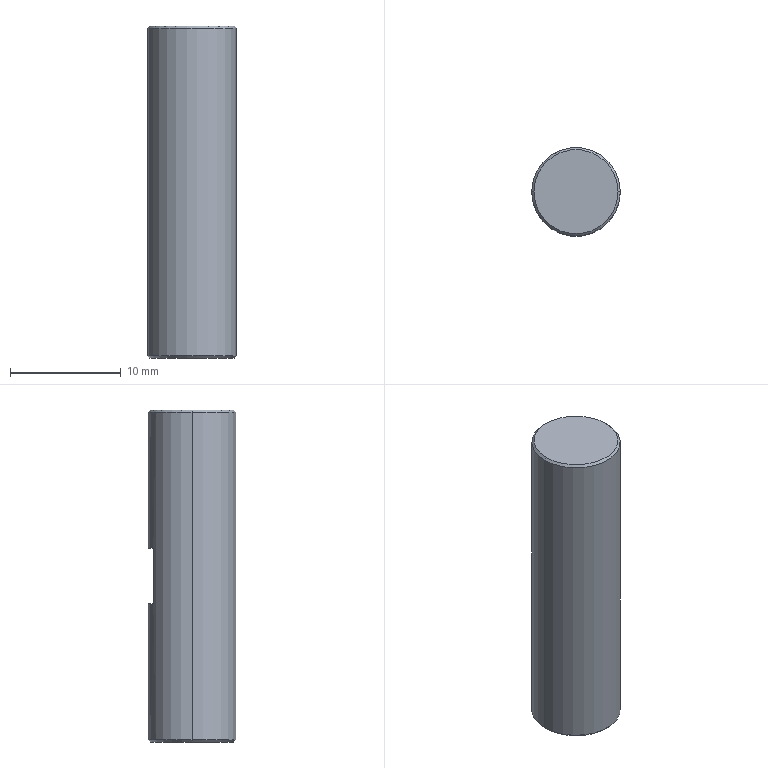Part | STEP file | 周轴^回墨刀-350 | 1 solid | 11 faces | box 8 x 8 x 30 mm | volume 1500 mm3 | plane 5 | cone 4 | cylinder 2 | commonest cylinder face diameters 8 x2
STEP:
#1=CARTESIAN_POINT('',(3.8,73.5,15.));
#2=VERTEX_POINT('',#1);
#3=CARTESIAN_POINT('',(-3.8,73.5,15.));
#4=VERTEX_POINT('',#3);
#5=CARTESIAN_POINT('',(0.,73.5,15.));
#6=DIRECTION('',(0.,0.,1.));
#7=DIRECTION('',(1.,0.,0.));
#8=AXIS2_PLACEMENT_3D('',#5,#6,#7);
#9=CIRCLE('',#8,3.8);
#10=EDGE_CURVE('',#2,#4,#9,.T.);
#11=ORIENTED_EDGE('',*,*,#10,.F.);
#12=CARTESIAN_POINT('',(4.,73.5,14.8));
#13=VERTEX_POINT('',#12);
#14=CARTESIAN_POINT('',(3.8,73.5,15.));
#15=DIRECTION('',(0.7071,0.,-0.7071));
#16=VECTOR('',#15,1000.);
#17=LINE('',#14,#16);
#18=EDGE_CURVE('',#2,#13,#17,.T.);
#19=ORIENTED_EDGE('',*,*,#18,.T.);
#20=CARTESIAN_POINT('',(-4.,73.5,14.8));
#21=VERTEX_POINT('',#20);
#22=CARTESIAN_POINT('',(0.,73.5,14.8));
#23=DIRECTION('',(0.,0.,-1.));
#24=DIRECTION('',(1.,0.,0.));
#25=AXIS2_PLACEMENT_3D('',#22,#23,#24);
#26=CIRCLE('',#25,4.);
#27=EDGE_CURVE('',#21,#13,#26,.T.);
#28=ORIENTED_EDGE('',*,*,#27,.F.);
#29=CARTESIAN_POINT('',(-3.8,73.5,15.));
#30=DIRECTION('',(-0.7071,0.,-0.7071));
#31=VECTOR('',#30,1000.);
#32=LINE('',#29,#31);
#33=EDGE_CURVE('',#4,#21,#32,.T.);
#34=ORIENTED_EDGE('',*,*,#33,.F.);
#35=EDGE_LOOP('',(#11,#19,#28,#34));
#36=FACE_OUTER_BOUND('',#35,.T.);
#37=CARTESIAN_POINT('',(0.,73.5,15.));
#38=DIRECTION('',(0.,0.,-1.));
#39=DIRECTION('',(-1.,0.,0.));
#40=AXIS2_PLACEMENT_3D('',#37,#38,#39);
#41=CONICAL_SURFACE('',#40,3.8,0.7854);
#42=ADVANCED_FACE('',(#36),#41,.T.);
#43=CARTESIAN_POINT('',(-3.8,73.5,-15.));
#44=VERTEX_POINT('',#43);
#45=CARTESIAN_POINT('',(3.8,73.5,-15.));
#46=VERTEX_POINT('',#45);
#47=CARTESIAN_POINT('',(0.,73.5,-15.));
#48=DIRECTION('',(0.,0.,-1.));
#49=DIRECTION('',(1.,0.,0.));
#50=AXIS2_PLACEMENT_3D('',#47,#48,#49);
#51=CIRCLE('',#50,3.8);
#52=EDGE_CURVE('',#44,#46,#51,.T.);
#53=ORIENTED_EDGE('',*,*,#52,.F.);
#54=CARTESIAN_POINT('',(-4.,73.5,-14.8));
#55=VERTEX_POINT('',#54);
#56=CARTESIAN_POINT('',(-3.8,73.5,-15.));
#57=DIRECTION('',(-0.7071,0.,0.7071));
#58=VECTOR('',#57,1000.);
#59=LINE('',#56,#58);
#60=EDGE_CURVE('',#44,#55,#59,.T.);
#61=ORIENTED_EDGE('',*,*,#60,.T.);
#62=CARTESIAN_POINT('',(4.,73.5,-14.8));
#63=VERTEX_POINT('',#62);
#64=CARTESIAN_POINT('',(0.,73.5,-14.8));
#65=DIRECTION('',(0.,0.,1.));
#66=DIRECTION('',(1.,0.,0.));
#67=AXIS2_PLACEMENT_3D('',#64,#65,#66);
#68=CIRCLE('',#67,4.);
#69=EDGE_CURVE('',#63,#55,#68,.T.);
#70=ORIENTED_EDGE('',*,*,#69,.F.);
#71=CARTESIAN_POINT('',(3.8,73.5,-15.));
#72=DIRECTION('',(0.7071,0.,0.7071));
#73=VECTOR('',#72,1000.);
#74=LINE('',#71,#73);
#75=EDGE_CURVE('',#46,#63,#74,.T.);
#76=ORIENTED_EDGE('',*,*,#75,.F.);
#77=EDGE_LOOP('',(#53,#61,#70,#76));
#78=FACE_OUTER_BOUND('',#77,.T.);
#79=CARTESIAN_POINT('',(0.,73.5,-15.));
#80=DIRECTION('',(0.,0.,1.));
#81=DIRECTION('',(1.,0.,0.));
#82=AXIS2_PLACEMENT_3D('',#79,#80,#81);
#83=CONICAL_SURFACE('',#82,3.8,0.7854);
#84=ADVANCED_FACE('',(#78),#83,.T.);
#85=CARTESIAN_POINT('',(-1.936,77.,-2.5));
#86=VERTEX_POINT('',#85);
#87=CARTESIAN_POINT('',(-1.936,77.,2.5));
#88=VERTEX_POINT('',#87);
#89=CARTESIAN_POINT('',(-1.936,77.,-26.314));
#90=DIRECTION('',(0.,0.,1.));
#91=VECTOR('',#90,1000.);
#92=LINE('',#89,#91);
#93=EDGE_CURVE('',#86,#88,#92,.T.);
#94=ORIENTED_EDGE('',*,*,#93,.F.);
#95=CARTESIAN_POINT('',(1.936,77.,-2.5));
#96=VERTEX_POINT('',#95);
#97=CARTESIAN_POINT('',(0.,73.5,-2.5));
#98=DIRECTION('',(0.,0.,-1.));
#99=DIRECTION('',(1.,0.,0.));
#100=AXIS2_PLACEMENT_3D('',#97,#98,#99);
#101=CIRCLE('',#100,4.);
#102=EDGE_CURVE('',#86,#96,#101,.T.);
#103=ORIENTED_EDGE('',*,*,#102,.T.);
#104=CARTESIAN_POINT('',(1.936,77.,2.5));
#105=VERTEX_POINT('',#104);
#106=CARTESIAN_POINT('',(1.936,77.,-26.314));
#107=DIRECTION('',(0.,0.,-1.));
#108=VECTOR('',#107,1000.);
#109=LINE('',#106,#108);
#110=EDGE_CURVE('',#105,#96,#109,.T.);
#111=ORIENTED_EDGE('',*,*,#110,.F.);
#112=CARTESIAN_POINT('',(0.,73.5,2.5));
#113=DIRECTION('',(0.,0.,-1.));
#114=DIRECTION('',(1.,0.,0.));
#115=AXIS2_PLACEMENT_3D('',#112,#113,#114);
#116=CIRCLE('',#115,4.);
#117=EDGE_CURVE('',#88,#105,#116,.T.);
#118=ORIENTED_EDGE('',*,*,#117,.F.);
#119=EDGE_LOOP('',(#94,#103,#111,#118));
#120=FACE_BOUND('',#119,.T.);
#121=ORIENTED_EDGE('',*,*,#69,.T.);
#122=CARTESIAN_POINT('',(-4.,73.5,-26.314));
#123=DIRECTION('',(0.,0.,1.));
#124=VECTOR('',#123,1000.);
#125=LINE('',#122,#124);
#126=EDGE_CURVE('',#55,#21,#125,.T.);
#127=ORIENTED_EDGE('',*,*,#126,.T.);
#128=ORIENTED_EDGE('',*,*,#27,.T.);
#129=CARTESIAN_POINT('',(4.,73.5,-26.314));
#130=DIRECTION('',(0.,0.,1.));
#131=VECTOR('',#130,1000.);
#132=LINE('',#129,#131);
#133=EDGE_CURVE('',#63,#13,#132,.T.);
#134=ORIENTED_EDGE('',*,*,#133,.F.);
#135=EDGE_LOOP('',(#121,#127,#128,#134));
#136=FACE_OUTER_BOUND('',#135,.T.);
#137=CARTESIAN_POINT('',(0.,73.5,-26.314));
#138=DIRECTION('',(0.,0.,1.));
#139=DIRECTION('',(1.,0.,0.));
#140=AXIS2_PLACEMENT_3D('',#137,#138,#139);
#141=CYLINDRICAL_SURFACE('',#140,4.);
#142=ADVANCED_FACE('',(#120,#136),#141,.T.);
#143=ORIENTED_EDGE('',*,*,#126,.F.);
#144=CARTESIAN_POINT('',(0.,73.5,-14.8));
#145=DIRECTION('',(0.,0.,1.));
#146=DIRECTION('',(1.,0.,0.));
#147=AXIS2_PLACEMENT_3D('',#144,#145,#146);
#148=CIRCLE('',#147,4.);
#149=EDGE_CURVE('',#55,#63,#148,.T.);
#150=ORIENTED_EDGE('',*,*,#149,.T.);
#151=ORIENTED_EDGE('',*,*,#133,.T.);
#152=CARTESIAN_POINT('',(0.,73.5,14.8));
#153=DIRECTION('',(0.,0.,-1.));
#154=DIRECTION('',(1.,0.,0.));
#155=AXIS2_PLACEMENT_3D('',#152,#153,#154);
#156=CIRCLE('',#155,4.);
#157=EDGE_CURVE('',#13,#21,#156,.T.);
#158=ORIENTED_EDGE('',*,*,#157,.T.);
#159=EDGE_LOOP('',(#143,#150,#151,#158));
#160=FACE_OUTER_BOUND('',#159,.T.);
#161=CARTESIAN_POINT('',(0.,73.5,-26.314));
#162=DIRECTION('',(0.,0.,1.));
#163=DIRECTION('',(1.,0.,0.));
#164=AXIS2_PLACEMENT_3D('',#161,#162,#163);
#165=CYLINDRICAL_SURFACE('',#164,4.);
#166=ADVANCED_FACE('',(#160),#165,.T.);
#167=CARTESIAN_POINT('',(0.,73.5,15.));
#168=DIRECTION('',(0.,0.,1.));
#169=DIRECTION('',(1.,0.,0.));
#170=AXIS2_PLACEMENT_3D('',#167,#168,#169);
#171=CIRCLE('',#170,3.8);
#172=EDGE_CURVE('',#4,#2,#171,.T.);
#173=ORIENTED_EDGE('',*,*,#172,.T.);
#174=ORIENTED_EDGE('',*,*,#10,.T.);
#175=EDGE_LOOP('',(#173,#174));
#176=FACE_OUTER_BOUND('',#175,.T.);
#177=CARTESIAN_POINT('',(0.,73.5,15.));
#178=DIRECTION('',(0.,0.,1.));
#179=DIRECTION('',(1.,0.,0.));
#180=AXIS2_PLACEMENT_3D('',#177,#178,#179);
#181=PLANE('',#180);
#182=ADVANCED_FACE('',(#176),#181,.T.);
#183=CARTESIAN_POINT('',(0.,73.5,-15.));
#184=DIRECTION('',(0.,0.,-1.));
#185=DIRECTION('',(1.,0.,0.));
#186=AXIS2_PLACEMENT_3D('',#183,#184,#185);
#187=CIRCLE('',#186,3.8);
#188=EDGE_CURVE('',#46,#44,#187,.T.);
#189=ORIENTED_EDGE('',*,*,#188,.T.);
#190=ORIENTED_EDGE('',*,*,#52,.T.);
#191=EDGE_LOOP('',(#189,#190));
#192=FACE_OUTER_BOUND('',#191,.T.);
#193=CARTESIAN_POINT('',(120.,84.5,-15.));
#194=DIRECTION('',(0.,0.,1.));
#195=DIRECTION('',(1.,0.,0.));
#196=AXIS2_PLACEMENT_3D('',#193,#194,#195);
#197=PLANE('',#196);
#198=ADVANCED_FACE('',(#192),#197,.F.);
#199=ORIENTED_EDGE('',*,*,#60,.F.);
#200=ORIENTED_EDGE('',*,*,#188,.F.);
#201=ORIENTED_EDGE('',*,*,#75,.T.);
#202=ORIENTED_EDGE('',*,*,#149,.F.);
#203=EDGE_LOOP('',(#199,#200,#201,#202));
#204=FACE_OUTER_BOUND('',#203,.T.);
#205=CARTESIAN_POINT('',(0.,73.5,-15.));
#206=DIRECTION('',(0.,0.,1.));
#207=DIRECTION('',(1.,0.,0.));
#208=AXIS2_PLACEMENT_3D('',#205,#206,#207);
#209=CONICAL_SURFACE('',#208,3.8,0.7854);
#210=ADVANCED_FACE('',(#204),#209,.T.);
#211=ORIENTED_EDGE('',*,*,#18,.F.);
#212=ORIENTED_EDGE('',*,*,#172,.F.);
#213=ORIENTED_EDGE('',*,*,#33,.T.);
#214=ORIENTED_EDGE('',*,*,#157,.F.);
#215=EDGE_LOOP('',(#211,#212,#213,#214));
#216=FACE_OUTER_BOUND('',#215,.T.);
#217=CARTESIAN_POINT('',(0.,73.5,15.));
#218=DIRECTION('',(0.,0.,-1.));
#219=DIRECTION('',(-1.,0.,0.));
#220=AXIS2_PLACEMENT_3D('',#217,#218,#219);
#221=CONICAL_SURFACE('',#220,3.8,0.7854);
#222=ADVANCED_FACE('',(#216),#221,.T.);
#223=ORIENTED_EDGE('',*,*,#110,.T.);
#224=CARTESIAN_POINT('',(-2.84,77.,-2.5));
#225=DIRECTION('',(1.,0.,0.));
#226=VECTOR('',#225,1000.);
#227=LINE('',#224,#226);
#228=EDGE_CURVE('',#86,#96,#227,.T.);
#229=ORIENTED_EDGE('',*,*,#228,.F.);
#230=ORIENTED_EDGE('',*,*,#93,.T.);
#231=CARTESIAN_POINT('',(-2.84,77.,2.5));
#232=DIRECTION('',(1.,0.,0.));
#233=VECTOR('',#232,1000.);
#234=LINE('',#231,#233);
#235=EDGE_CURVE('',#88,#105,#234,.T.);
#236=ORIENTED_EDGE('',*,*,#235,.T.);
#237=EDGE_LOOP('',(#223,#229,#230,#236));
#238=FACE_OUTER_BOUND('',#237,.T.);
#239=CARTESIAN_POINT('',(-2.84,77.,-2.5));
#240=DIRECTION('',(0.,-1.,0.));
#241=DIRECTION('',(0.,0.,-1.));
#242=AXIS2_PLACEMENT_3D('',#239,#240,#241);
#243=PLANE('',#242);
#244=ADVANCED_FACE('',(#238),#243,.F.);
#245=ORIENTED_EDGE('',*,*,#228,.T.);
#246=ORIENTED_EDGE('',*,*,#102,.F.);
#247=EDGE_LOOP('',(#245,#246));
#248=FACE_OUTER_BOUND('',#247,.T.);
#249=CARTESIAN_POINT('',(-2.84,77.,-2.5));
#250=DIRECTION('',(0.,0.,1.));
#251=DIRECTION('',(1.,0.,0.));
#252=AXIS2_PLACEMENT_3D('',#249,#250,#251);
#253=PLANE('',#252);
#254=ADVANCED_FACE('',(#248),#253,.T.);
#255=ORIENTED_EDGE('',*,*,#117,.T.);
#256=ORIENTED_EDGE('',*,*,#235,.F.);
#257=EDGE_LOOP('',(#255,#256));
#258=FACE_OUTER_BOUND('',#257,.T.);
#259=CARTESIAN_POINT('',(-2.84,77.,2.5));
#260=DIRECTION('',(0.,0.,1.));
#261=DIRECTION('',(1.,0.,0.));
#262=AXIS2_PLACEMENT_3D('',#259,#260,#261);
#263=PLANE('',#262);
#264=ADVANCED_FACE('',(#258),#263,.F.);
#265=CLOSED_SHELL('',(#42,#84,#142,#166,#182,#198,#210,#222,#244,#254,#264));
#266=MANIFOLD_SOLID_BREP('',#265);
#267=CARTESIAN_POINT('',(0.,0.,0.));
#268=DIRECTION('',(0.,0.,1.));
#269=DIRECTION('',(1.,0.,0.));
#270=AXIS2_PLACEMENT_3D('',#267,#268,#269);
#271=(LENGTH_UNIT()NAMED_UNIT(*)SI_UNIT(.MILLI.,.METRE.));
#272=UNCERTAINTY_MEASURE_WITH_UNIT(LENGTH_MEASURE(0.00001),#271,'','');
#273=(NAMED_UNIT(*)PLANE_ANGLE_UNIT()SI_UNIT($,.RADIAN.));
#274=(NAMED_UNIT(*)SI_UNIT($,.STERADIAN.)SOLID_ANGLE_UNIT());
#275=(GEOMETRIC_REPRESENTATION_CONTEXT(3)GLOBAL_UNCERTAINTY_ASSIGNED_CONTEXT((#272))GLOBAL_UNIT_ASSIGNED_CONTEXT((#271,#273,#274))REPRESENTATION_CONTEXT('',''));
#276=ADVANCED_BREP_SHAPE_REPRESENTATION('',(#266,#270),#275);